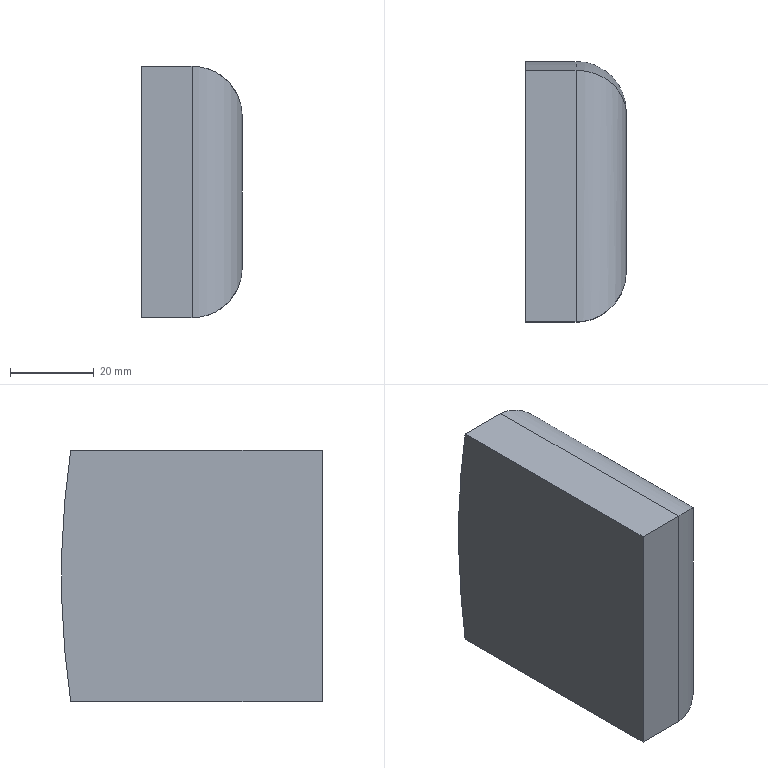Part | NX | 1 solid | 10 faces | box 24 x 62.191 x 60 mm | volume 81725 mm3 | plane 5 | cylinder 4 | torus 1 | commonest cylinder face diameters 24 x3 412.996 x1
STEP:
#1=CARTESIAN_POINT('',(280.674,-616.727,2398.086));
#2=VERTEX_POINT('',#1);
#3=CARTESIAN_POINT('',(268.674,-616.727,2398.086));
#4=VERTEX_POINT('',#3);
#5=CARTESIAN_POINT('',(292.674,-616.727,2398.086));
#6=DIRECTION('',(-1.,0.,0.));
#7=VECTOR('',#6,1.);
#8=LINE('',#5,#7);
#9=EDGE_CURVE('',#2,#4,#8,.T.);
#10=ORIENTED_EDGE('',*,*,#9,.T.);
#11=CARTESIAN_POINT('',(268.674,-616.727,2458.086));
#12=VERTEX_POINT('',#11);
#13=CARTESIAN_POINT('',(268.674,-821.034,2428.086));
#14=DIRECTION('',(-1.,0.,0.));
#15=DIRECTION('',(0.,0.,-1.));
#16=AXIS2_PLACEMENT_3D('',#13,#14,#15);
#17=CIRCLE('',#16,206.498);
#18=EDGE_CURVE('',#12,#4,#17,.T.);
#19=ORIENTED_EDGE('',*,*,#18,.F.);
#20=CARTESIAN_POINT('',(280.674,-616.727,2458.086));
#21=VERTEX_POINT('',#20);
#22=CARTESIAN_POINT('',(292.674,-616.727,2458.086));
#23=DIRECTION('',(-1.,0.,0.));
#24=VECTOR('',#23,1.);
#25=LINE('',#22,#24);
#26=EDGE_CURVE('',#21,#12,#25,.T.);
#27=ORIENTED_EDGE('',*,*,#26,.F.);
#28=CARTESIAN_POINT('',(280.674,-821.034,2428.086));
#29=DIRECTION('',(1.,0.,0.));
#30=DIRECTION('',(0.,0.,-1.));
#31=AXIS2_PLACEMENT_3D('',#28,#29,#30);
#32=CIRCLE('',#31,206.498);
#33=EDGE_CURVE('',#2,#21,#32,.T.);
#34=ORIENTED_EDGE('',*,*,#33,.F.);
#35=EDGE_LOOP('',(#10,#19,#27,#34));
#36=FACE_OUTER_BOUND('',#35,.T.);
#37=CARTESIAN_POINT('',(292.674,-821.034,2428.086));
#38=DIRECTION('',(-1.,0.,0.));
#39=DIRECTION('',(0.,0.,-1.));
#40=AXIS2_PLACEMENT_3D('',#37,#38,#39);
#41=CYLINDRICAL_SURFACE('',#40,206.498);
#42=ADVANCED_FACE('',(#36),#41,.T.);
#43=CARTESIAN_POINT('',(280.674,-676.727,2398.086));
#44=VERTEX_POINT('',#43);
#45=CARTESIAN_POINT('',(268.674,-676.727,2398.086));
#46=VERTEX_POINT('',#45);
#47=CARTESIAN_POINT('',(292.674,-676.727,2398.086));
#48=DIRECTION('',(-1.,0.,0.));
#49=VECTOR('',#48,1.);
#50=LINE('',#47,#49);
#51=EDGE_CURVE('',#44,#46,#50,.T.);
#52=ORIENTED_EDGE('',*,*,#51,.T.);
#53=CARTESIAN_POINT('',(268.674,-616.727,2398.086));
#54=DIRECTION('',(0.,-1.,0.));
#55=VECTOR('',#54,1.);
#56=LINE('',#53,#55);
#57=EDGE_CURVE('',#4,#46,#56,.T.);
#58=ORIENTED_EDGE('',*,*,#57,.F.);
#59=ORIENTED_EDGE('',*,*,#9,.F.);
#60=CARTESIAN_POINT('',(280.674,-616.727,2398.086));
#61=DIRECTION('',(0.,1.,0.));
#62=VECTOR('',#61,1.);
#63=LINE('',#60,#62);
#64=EDGE_CURVE('',#44,#2,#63,.T.);
#65=ORIENTED_EDGE('',*,*,#64,.F.);
#66=EDGE_LOOP('',(#52,#58,#59,#65));
#67=FACE_OUTER_BOUND('',#66,.T.);
#68=CARTESIAN_POINT('',(292.674,-616.727,2398.086));
#69=DIRECTION('',(0.,0.,1.));
#70=DIRECTION('',(0.,-1.,0.));
#71=AXIS2_PLACEMENT_3D('',#68,#69,#70);
#72=PLANE('',#71);
#73=ADVANCED_FACE('',(#67),#72,.F.);
#74=CARTESIAN_POINT('',(280.674,-676.727,2458.086));
#75=VERTEX_POINT('',#74);
#76=CARTESIAN_POINT('',(268.674,-676.727,2458.086));
#77=VERTEX_POINT('',#76);
#78=CARTESIAN_POINT('',(292.674,-676.727,2458.086));
#79=DIRECTION('',(-1.,0.,0.));
#80=VECTOR('',#79,1.);
#81=LINE('',#78,#80);
#82=EDGE_CURVE('',#75,#77,#81,.T.);
#83=ORIENTED_EDGE('',*,*,#82,.T.);
#84=CARTESIAN_POINT('',(268.674,-676.727,2398.086));
#85=DIRECTION('',(0.,0.,1.));
#86=VECTOR('',#85,1.);
#87=LINE('',#84,#86);
#88=EDGE_CURVE('',#46,#77,#87,.T.);
#89=ORIENTED_EDGE('',*,*,#88,.F.);
#90=ORIENTED_EDGE('',*,*,#51,.F.);
#91=CARTESIAN_POINT('',(280.674,-676.727,2398.086));
#92=DIRECTION('',(0.,0.,-1.));
#93=VECTOR('',#92,1.);
#94=LINE('',#91,#93);
#95=EDGE_CURVE('',#75,#44,#94,.T.);
#96=ORIENTED_EDGE('',*,*,#95,.F.);
#97=EDGE_LOOP('',(#83,#89,#90,#96));
#98=FACE_OUTER_BOUND('',#97,.T.);
#99=CARTESIAN_POINT('',(292.674,-676.727,2398.086));
#100=DIRECTION('',(0.,1.,0.));
#101=DIRECTION('',(0.,0.,1.));
#102=AXIS2_PLACEMENT_3D('',#99,#100,#101);
#103=PLANE('',#102);
#104=ADVANCED_FACE('',(#98),#103,.F.);
#105=ORIENTED_EDGE('',*,*,#26,.T.);
#106=CARTESIAN_POINT('',(268.674,-616.727,2458.086));
#107=DIRECTION('',(0.,1.,0.));
#108=VECTOR('',#107,1.);
#109=LINE('',#106,#108);
#110=EDGE_CURVE('',#77,#12,#109,.T.);
#111=ORIENTED_EDGE('',*,*,#110,.F.);
#112=ORIENTED_EDGE('',*,*,#82,.F.);
#113=CARTESIAN_POINT('',(280.674,-616.727,2458.086));
#114=DIRECTION('',(0.,-1.,0.));
#115=VECTOR('',#114,1.);
#116=LINE('',#113,#115);
#117=EDGE_CURVE('',#21,#75,#116,.T.);
#118=ORIENTED_EDGE('',*,*,#117,.F.);
#119=EDGE_LOOP('',(#105,#111,#112,#118));
#120=FACE_OUTER_BOUND('',#119,.T.);
#121=CARTESIAN_POINT('',(292.674,-616.727,2458.086));
#122=DIRECTION('',(0.,0.,-1.));
#123=DIRECTION('',(0.,1.,0.));
#124=AXIS2_PLACEMENT_3D('',#121,#122,#123);
#125=PLANE('',#124);
#126=ADVANCED_FACE('',(#120),#125,.F.);
#127=CARTESIAN_POINT('',(292.674,-664.727,2410.086));
#128=VERTEX_POINT('',#127);
#129=CARTESIAN_POINT('',(292.674,-664.727,2446.086));
#130=VERTEX_POINT('',#129);
#131=CARTESIAN_POINT('',(292.674,-664.727,2428.086));
#132=DIRECTION('',(0.,0.,1.));
#133=VECTOR('',#132,1.);
#134=LINE('',#131,#133);
#135=EDGE_CURVE('',#128,#130,#134,.T.);
#136=ORIENTED_EDGE('',*,*,#135,.F.);
#137=CARTESIAN_POINT('',(292.674,-627.371,2410.086));
#138=VERTEX_POINT('',#137);
#139=CARTESIAN_POINT('',(292.674,-821.034,2410.086));
#140=DIRECTION('',(0.,-1.,0.));
#141=VECTOR('',#140,1.);
#142=LINE('',#139,#141);
#143=EDGE_CURVE('',#138,#128,#142,.T.);
#144=ORIENTED_EDGE('',*,*,#143,.F.);
#145=CARTESIAN_POINT('',(292.674,-627.371,2446.086));
#146=VERTEX_POINT('',#145);
#147=CARTESIAN_POINT('',(292.674,-821.034,2428.086));
#148=DIRECTION('',(-1.,0.,0.));
#149=DIRECTION('',(0.,0.,-1.));
#150=AXIS2_PLACEMENT_3D('',#147,#148,#149);
#151=CIRCLE('',#150,194.498);
#152=EDGE_CURVE('',#146,#138,#151,.T.);
#153=ORIENTED_EDGE('',*,*,#152,.F.);
#154=CARTESIAN_POINT('',(292.674,-821.034,2446.086));
#155=DIRECTION('',(0.,1.,0.));
#156=VECTOR('',#155,1.);
#157=LINE('',#154,#156);
#158=EDGE_CURVE('',#130,#146,#157,.T.);
#159=ORIENTED_EDGE('',*,*,#158,.F.);
#160=EDGE_LOOP('',(#136,#144,#153,#159));
#161=FACE_OUTER_BOUND('',#160,.T.);
#162=CARTESIAN_POINT('',(292.674,-821.034,2428.086));
#163=DIRECTION('',(-1.,0.,0.));
#164=DIRECTION('',(0.,0.,-1.));
#165=AXIS2_PLACEMENT_3D('',#162,#163,#164);
#166=PLANE('',#165);
#167=ADVANCED_FACE('',(#161),#166,.F.);
#168=ORIENTED_EDGE('',*,*,#18,.T.);
#169=ORIENTED_EDGE('',*,*,#57,.T.);
#170=ORIENTED_EDGE('',*,*,#88,.T.);
#171=ORIENTED_EDGE('',*,*,#110,.T.);
#172=EDGE_LOOP('',(#168,#169,#170,#171));
#173=FACE_OUTER_BOUND('',#172,.T.);
#174=CARTESIAN_POINT('',(268.674,-821.034,2428.086));
#175=DIRECTION('',(-1.,0.,0.));
#176=DIRECTION('',(0.,0.,-1.));
#177=AXIS2_PLACEMENT_3D('',#174,#175,#176);
#178=PLANE('',#177);
#179=ADVANCED_FACE('',(#173),#178,.T.);
#180=CARTESIAN_POINT('',(280.674,-616.727,2398.086));
#181=CARTESIAN_POINT('',(282.543,-616.727,2398.086));
#182=CARTESIAN_POINT('',(284.356,-617.114,2398.535));
#183=CARTESIAN_POINT('',(287.464,-618.423,2400.042));
#184=CARTESIAN_POINT('',(288.749,-619.324,2401.076));
#185=CARTESIAN_POINT('',(291.783,-622.417,2404.593));
#186=CARTESIAN_POINT('',(292.674,-624.893,2407.368));
#187=CARTESIAN_POINT('',(292.674,-627.371,2410.086));
#188=B_SPLINE_CURVE_WITH_KNOTS('',3,(#180,#181,#182,#183,#184,#185,#186,#187),.UNSPECIFIED.,.F.,.F.,(4,2,2,4),(0.,0.25,0.5,1.),.UNSPECIFIED.);
#189=EDGE_CURVE('',#2,#138,#188,.T.);
#190=ORIENTED_EDGE('',*,*,#189,.T.);
#191=ORIENTED_EDGE('',*,*,#143,.T.);
#192=CARTESIAN_POINT('',(292.674,-664.727,2410.086));
#193=CARTESIAN_POINT('',(292.674,-671.756,2403.057));
#194=CARTESIAN_POINT('',(287.703,-676.727,2398.086));
#195=CARTESIAN_POINT('',(280.674,-676.727,2398.086));
#196=(BOUNDED_CURVE()B_SPLINE_CURVE(3,(#192,#193,#194,#195),.UNSPECIFIED.,.F.,.F.)B_SPLINE_CURVE_WITH_KNOTS((4,4),(0.,1.),.UNSPECIFIED.)CURVE()GEOMETRIC_REPRESENTATION_ITEM()RATIONAL_B_SPLINE_CURVE((1.,0.8047,0.8047,1.))REPRESENTATION_ITEM(''));
#197=EDGE_CURVE('',#128,#44,#196,.T.);
#198=ORIENTED_EDGE('',*,*,#197,.T.);
#199=ORIENTED_EDGE('',*,*,#64,.T.);
#200=EDGE_LOOP('',(#190,#191,#198,#199));
#201=FACE_OUTER_BOUND('',#200,.T.);
#202=CARTESIAN_POINT('',(280.674,-821.034,2410.086));
#203=DIRECTION('',(0.,-1.,0.));
#204=DIRECTION('',(0.,0.,-1.));
#205=AXIS2_PLACEMENT_3D('',#202,#203,#204);
#206=CYLINDRICAL_SURFACE('',#205,12.);
#207=ADVANCED_FACE('',(#201),#206,.T.);
#208=ORIENTED_EDGE('',*,*,#197,.F.);
#209=ORIENTED_EDGE('',*,*,#135,.T.);
#210=CARTESIAN_POINT('',(292.674,-664.727,2446.086));
#211=CARTESIAN_POINT('',(292.674,-671.756,2453.116));
#212=CARTESIAN_POINT('',(287.703,-676.727,2458.086));
#213=CARTESIAN_POINT('',(280.674,-676.727,2458.086));
#214=(BOUNDED_CURVE()B_SPLINE_CURVE(3,(#210,#211,#212,#213),.UNSPECIFIED.,.F.,.F.)B_SPLINE_CURVE_WITH_KNOTS((4,4),(0.,1.),.UNSPECIFIED.)CURVE()GEOMETRIC_REPRESENTATION_ITEM()RATIONAL_B_SPLINE_CURVE((1.,0.8047,0.8047,1.))REPRESENTATION_ITEM(''));
#215=EDGE_CURVE('',#130,#75,#214,.T.);
#216=ORIENTED_EDGE('',*,*,#215,.T.);
#217=ORIENTED_EDGE('',*,*,#95,.T.);
#218=EDGE_LOOP('',(#208,#209,#216,#217));
#219=FACE_OUTER_BOUND('',#218,.T.);
#220=CARTESIAN_POINT('',(280.674,-664.727,2428.086));
#221=DIRECTION('',(0.,0.,1.));
#222=DIRECTION('',(-1.,0.,0.));
#223=AXIS2_PLACEMENT_3D('',#220,#221,#222);
#224=CYLINDRICAL_SURFACE('',#223,12.);
#225=ADVANCED_FACE('',(#219),#224,.T.);
#226=ORIENTED_EDGE('',*,*,#189,.F.);
#227=ORIENTED_EDGE('',*,*,#33,.T.);
#228=CARTESIAN_POINT('',(280.674,-616.727,2458.086));
#229=CARTESIAN_POINT('',(282.543,-616.727,2458.086));
#230=CARTESIAN_POINT('',(284.356,-617.114,2457.637));
#231=CARTESIAN_POINT('',(287.464,-618.423,2456.13));
#232=CARTESIAN_POINT('',(288.749,-619.324,2455.097));
#233=CARTESIAN_POINT('',(291.783,-622.417,2451.58));
#234=CARTESIAN_POINT('',(292.674,-624.893,2448.805));
#235=CARTESIAN_POINT('',(292.674,-627.371,2446.086));
#236=B_SPLINE_CURVE_WITH_KNOTS('',3,(#228,#229,#230,#231,#232,#233,#234,#235),.UNSPECIFIED.,.F.,.F.,(4,2,2,4),(0.,0.25,0.5,1.),.UNSPECIFIED.);
#237=EDGE_CURVE('',#21,#146,#236,.T.);
#238=ORIENTED_EDGE('',*,*,#237,.T.);
#239=ORIENTED_EDGE('',*,*,#152,.T.);
#240=EDGE_LOOP('',(#226,#227,#238,#239));
#241=FACE_OUTER_BOUND('',#240,.T.);
#242=CARTESIAN_POINT('',(280.674,-821.034,2428.086));
#243=DIRECTION('',(-1.,0.,0.));
#244=DIRECTION('',(0.,0.,-1.));
#245=AXIS2_PLACEMENT_3D('',#242,#243,#244);
#246=TOROIDAL_SURFACE('',#245,194.498,12.);
#247=ADVANCED_FACE('',(#241),#246,.T.);
#248=ORIENTED_EDGE('',*,*,#215,.F.);
#249=ORIENTED_EDGE('',*,*,#158,.T.);
#250=ORIENTED_EDGE('',*,*,#237,.F.);
#251=ORIENTED_EDGE('',*,*,#117,.T.);
#252=EDGE_LOOP('',(#248,#249,#250,#251));
#253=FACE_OUTER_BOUND('',#252,.T.);
#254=CARTESIAN_POINT('',(280.674,-821.034,2446.086));
#255=DIRECTION('',(0.,1.,0.));
#256=DIRECTION('',(0.,0.,1.));
#257=AXIS2_PLACEMENT_3D('',#254,#255,#256);
#258=CYLINDRICAL_SURFACE('',#257,12.);
#259=ADVANCED_FACE('',(#253),#258,.T.);
#260=CLOSED_SHELL('',(#42,#73,#104,#126,#167,#179,#207,#225,#247,#259));
#261=MANIFOLD_SOLID_BREP('',#260);
#262=(LENGTH_UNIT()NAMED_UNIT(*)SI_UNIT(.MILLI.,.METRE.));
#263=UNCERTAINTY_MEASURE_WITH_UNIT(LENGTH_MEASURE(0.0508),#262,'','');
#264=(NAMED_UNIT(*)PLANE_ANGLE_UNIT()SI_UNIT($,.RADIAN.));
#265=PLANE_ANGLE_MEASURE_WITH_UNIT(PLANE_ANGLE_MEASURE(0.01745),#264);
#266=DIMENSIONAL_EXPONENTS(0.,0.,0.,0.,0.,0.,0.);
#267=(CONVERSION_BASED_UNIT('DEGREE',#265)NAMED_UNIT(#266)PLANE_ANGLE_UNIT());
#268=(NAMED_UNIT(*)SI_UNIT($,.STERADIAN.)SOLID_ANGLE_UNIT());
#269=(GEOMETRIC_REPRESENTATION_CONTEXT(3)GLOBAL_UNCERTAINTY_ASSIGNED_CONTEXT((#263))GLOBAL_UNIT_ASSIGNED_CONTEXT((#262,#267,#268))REPRESENTATION_CONTEXT('',''));
#270=ADVANCED_BREP_SHAPE_REPRESENTATION('',(#261),#269);